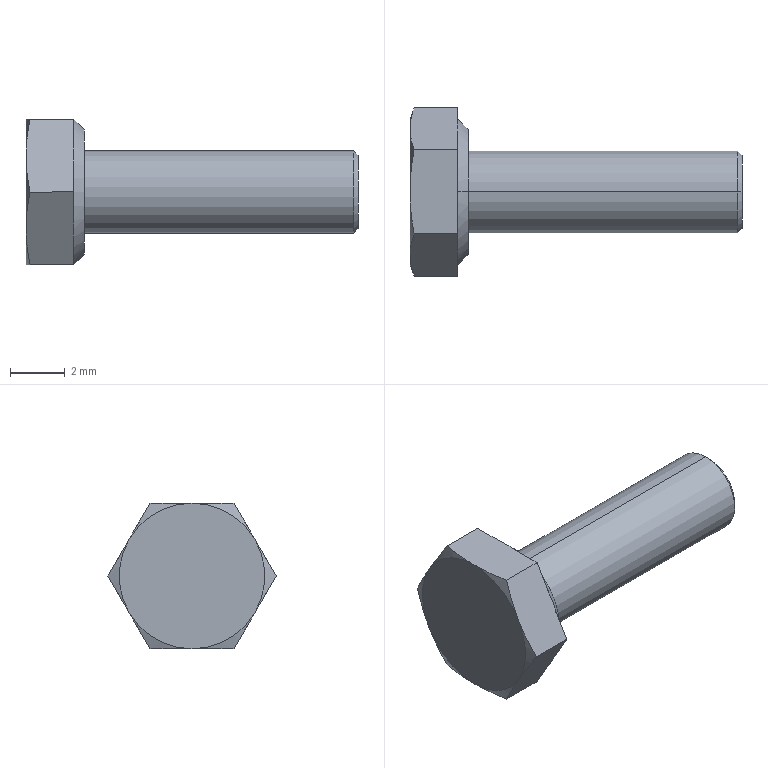Part | SolidWorks | features RevCut 3, Boss 1, Chamfer 1, Extrusion 1, Fillet 1, LPattern 1 | 1 solid | 27 faces | box 12.125 x 6.143 x 5.32 mm | volume 120.535 mm3 | plane 15 | cone 10 | cylinder 2 | commonest cylinder face diameters 3 x2
STEP:
#1=CARTESIAN_POINT('',(12.125,0.,-1.35));
#2=VERTEX_POINT('',#1);
#3=CARTESIAN_POINT('',(12.125,0.,1.35));
#4=VERTEX_POINT('',#3);
#5=CARTESIAN_POINT('',(12.125,0.,0.));
#6=DIRECTION('',(1.,0.,0.));
#7=DIRECTION('',(0.,0.,-1.));
#8=AXIS2_PLACEMENT_3D('',#5,#6,#7);
#9=CIRCLE('',#8,1.35);
#10=EDGE_CURVE('',#2,#4,#9,.T.);
#11=ORIENTED_EDGE('',*,*,#10,.F.);
#12=CARTESIAN_POINT('',(11.975,0.,-1.5));
#13=VERTEX_POINT('',#12);
#14=CARTESIAN_POINT('',(12.125,0.,-1.35));
#15=DIRECTION('',(-0.7071,0.,-0.7071));
#16=VECTOR('',#15,1000.);
#17=LINE('',#14,#16);
#18=EDGE_CURVE('',#2,#13,#17,.T.);
#19=ORIENTED_EDGE('',*,*,#18,.T.);
#20=CARTESIAN_POINT('',(11.975,0.,1.5));
#21=VERTEX_POINT('',#20);
#22=CARTESIAN_POINT('',(11.975,0.,0.));
#23=DIRECTION('',(-1.,0.,0.));
#24=DIRECTION('',(0.,0.,-1.));
#25=AXIS2_PLACEMENT_3D('',#22,#23,#24);
#26=CIRCLE('',#25,1.5);
#27=EDGE_CURVE('',#21,#13,#26,.T.);
#28=ORIENTED_EDGE('',*,*,#27,.F.);
#29=CARTESIAN_POINT('',(12.125,0.,1.35));
#30=DIRECTION('',(-0.7071,0.,0.7071));
#31=VECTOR('',#30,1000.);
#32=LINE('',#29,#31);
#33=EDGE_CURVE('',#4,#21,#32,.T.);
#34=ORIENTED_EDGE('',*,*,#33,.F.);
#35=EDGE_LOOP('',(#11,#19,#28,#34));
#36=FACE_OUTER_BOUND('',#35,.T.);
#37=CARTESIAN_POINT('',(12.125,0.,0.));
#38=DIRECTION('',(-1.,0.,0.));
#39=DIRECTION('',(0.,0.,1.));
#40=AXIS2_PLACEMENT_3D('',#37,#38,#39);
#41=CONICAL_SURFACE('',#40,1.35,0.7854);
#42=ADVANCED_FACE('',(#36),#41,.T.);
#43=ORIENTED_EDGE('',*,*,#27,.T.);
#44=CARTESIAN_POINT('',(2.125,0.,-1.5));
#45=VERTEX_POINT('',#44);
#46=CARTESIAN_POINT('',(12.125,0.,-1.5));
#47=DIRECTION('',(-1.,0.,0.));
#48=VECTOR('',#47,1000.);
#49=LINE('',#46,#48);
#50=EDGE_CURVE('',#13,#45,#49,.T.);
#51=ORIENTED_EDGE('',*,*,#50,.T.);
#52=CARTESIAN_POINT('',(2.125,0.,1.5));
#53=VERTEX_POINT('',#52);
#54=CARTESIAN_POINT('',(2.125,0.,0.));
#55=DIRECTION('',(1.,0.,0.));
#56=DIRECTION('',(0.,0.,-1.));
#57=AXIS2_PLACEMENT_3D('',#54,#55,#56);
#58=CIRCLE('',#57,1.5);
#59=EDGE_CURVE('',#45,#53,#58,.T.);
#60=ORIENTED_EDGE('',*,*,#59,.T.);
#61=CARTESIAN_POINT('',(12.125,0.,1.5));
#62=DIRECTION('',(-1.,0.,0.));
#63=VECTOR('',#62,1000.);
#64=LINE('',#61,#63);
#65=EDGE_CURVE('',#21,#53,#64,.T.);
#66=ORIENTED_EDGE('',*,*,#65,.F.);
#67=EDGE_LOOP('',(#43,#51,#60,#66));
#68=FACE_OUTER_BOUND('',#67,.T.);
#69=CARTESIAN_POINT('',(12.125,0.,0.));
#70=DIRECTION('',(-1.,0.,0.));
#71=DIRECTION('',(0.,0.,1.));
#72=AXIS2_PLACEMENT_3D('',#69,#70,#71);
#73=CYLINDRICAL_SURFACE('',#72,1.5);
#74=ADVANCED_FACE('',(#68),#73,.T.);
#75=CARTESIAN_POINT('',(2.125,0.,2.285));
#76=VERTEX_POINT('',#75);
#77=CARTESIAN_POINT('',(2.125,0.,-2.285));
#78=VERTEX_POINT('',#77);
#79=CARTESIAN_POINT('',(2.125,0.,0.));
#80=DIRECTION('',(-1.,0.,0.));
#81=DIRECTION('',(0.,0.,1.));
#82=AXIS2_PLACEMENT_3D('',#79,#80,#81);
#83=CIRCLE('',#82,2.285);
#84=EDGE_CURVE('',#76,#78,#83,.T.);
#85=ORIENTED_EDGE('',*,*,#84,.T.);
#86=CARTESIAN_POINT('',(1.75,0.,-2.66));
#87=VERTEX_POINT('',#86);
#88=CARTESIAN_POINT('',(1.725,0.,-2.685));
#89=DIRECTION('',(-0.7071,0.,-0.7071));
#90=VECTOR('',#89,1000.);
#91=LINE('',#88,#90);
#92=EDGE_CURVE('',#78,#87,#91,.T.);
#93=ORIENTED_EDGE('',*,*,#92,.T.);
#94=CARTESIAN_POINT('',(1.725,0.3655,-2.66));
#95=VERTEX_POINT('',#94);
#96=CARTESIAN_POINT('',(1.75,0.,-2.66));
#97=CARTESIAN_POINT('',(1.75,0.122,-2.66));
#98=CARTESIAN_POINT('',(1.742,0.2438,-2.66));
#99=CARTESIAN_POINT('',(1.725,0.3655,-2.66));
#100=B_SPLINE_CURVE_WITH_KNOTS('',3,(#96,#97,#98,#99),.UNSPECIFIED.,.F.,.F.,(4,4),(0.005987,0.006353),.UNSPECIFIED.);
#101=EDGE_CURVE('',#87,#95,#100,.T.);
#102=ORIENTED_EDGE('',*,*,#101,.T.);
#103=CARTESIAN_POINT('',(1.725,2.121,-1.647));
#104=VERTEX_POINT('',#103);
#105=CARTESIAN_POINT('',(1.725,0.,0.));
#106=DIRECTION('',(-1.,0.,0.));
#107=DIRECTION('',(0.,0.,1.));
#108=AXIS2_PLACEMENT_3D('',#105,#106,#107);
#109=CIRCLE('',#108,2.685);
#110=EDGE_CURVE('',#104,#95,#109,.T.);
#111=ORIENTED_EDGE('',*,*,#110,.F.);
#112=CARTESIAN_POINT('',(1.725,2.486,-1.013));
#113=VERTEX_POINT('',#112);
#114=CARTESIAN_POINT('',(1.725,2.121,-1.647));
#115=CARTESIAN_POINT('',(1.758,2.243,-1.436));
#116=CARTESIAN_POINT('',(1.758,2.365,-1.224));
#117=CARTESIAN_POINT('',(1.725,2.486,-1.013));
#118=B_SPLINE_CURVE_WITH_KNOTS('',3,(#114,#115,#116,#117),.UNSPECIFIED.,.F.,.F.,(4,4),(0.000001466,0.0007326),.UNSPECIFIED.);
#119=EDGE_CURVE('',#104,#113,#118,.T.);
#120=ORIENTED_EDGE('',*,*,#119,.T.);
#121=CARTESIAN_POINT('',(1.725,2.486,1.013));
#122=VERTEX_POINT('',#121);
#123=CARTESIAN_POINT('',(1.725,0.,0.));
#124=DIRECTION('',(-1.,0.,0.));
#125=DIRECTION('',(0.,0.,1.));
#126=AXIS2_PLACEMENT_3D('',#123,#124,#125);
#127=CIRCLE('',#126,2.685);
#128=EDGE_CURVE('',#122,#113,#127,.T.);
#129=ORIENTED_EDGE('',*,*,#128,.F.);
#130=CARTESIAN_POINT('',(1.725,2.121,1.647));
#131=VERTEX_POINT('',#130);
#132=CARTESIAN_POINT('',(1.725,2.486,1.013));
#133=CARTESIAN_POINT('',(1.758,2.365,1.224));
#134=CARTESIAN_POINT('',(1.758,2.243,1.436));
#135=CARTESIAN_POINT('',(1.725,2.121,1.647));
#136=B_SPLINE_CURVE_WITH_KNOTS('',3,(#132,#133,#134,#135),.UNSPECIFIED.,.F.,.F.,(4,4),(0.000001466,0.0007326),.UNSPECIFIED.);
#137=EDGE_CURVE('',#122,#131,#136,.T.);
#138=ORIENTED_EDGE('',*,*,#137,.T.);
#139=CARTESIAN_POINT('',(1.725,0.3655,2.66));
#140=VERTEX_POINT('',#139);
#141=CARTESIAN_POINT('',(1.725,0.,0.));
#142=DIRECTION('',(-1.,0.,0.));
#143=DIRECTION('',(0.,0.,1.));
#144=AXIS2_PLACEMENT_3D('',#141,#142,#143);
#145=CIRCLE('',#144,2.685);
#146=EDGE_CURVE('',#140,#131,#145,.T.);
#147=ORIENTED_EDGE('',*,*,#146,.F.);
#148=CARTESIAN_POINT('',(1.75,0.,2.66));
#149=VERTEX_POINT('',#148);
#150=CARTESIAN_POINT('',(1.725,0.3655,2.66));
#151=CARTESIAN_POINT('',(1.741,0.2453,2.66));
#152=CARTESIAN_POINT('',(1.75,0.1222,2.66));
#153=CARTESIAN_POINT('',(1.75,0.,2.66));
#154=B_SPLINE_CURVE_WITH_KNOTS('',3,(#150,#151,#152,#153),.UNSPECIFIED.,.F.,.F.,(4,4),(0.001277,0.001636),.UNSPECIFIED.);
#155=EDGE_CURVE('',#140,#149,#154,.T.);
#156=ORIENTED_EDGE('',*,*,#155,.T.);
#157=CARTESIAN_POINT('',(1.725,0.,2.685));
#158=DIRECTION('',(-0.7071,0.,0.7071));
#159=VECTOR('',#158,1000.);
#160=LINE('',#157,#159);
#161=EDGE_CURVE('',#76,#149,#160,.T.);
#162=ORIENTED_EDGE('',*,*,#161,.F.);
#163=EDGE_LOOP('',(#85,#93,#102,#111,#120,#129,#138,#147,#156,#162));
#164=FACE_OUTER_BOUND('',#163,.T.);
#165=CARTESIAN_POINT('',(1.725,0.,0.));
#166=DIRECTION('',(-1.,0.,0.));
#167=DIRECTION('',(0.,0.,1.));
#168=AXIS2_PLACEMENT_3D('',#165,#166,#167);
#169=CONICAL_SURFACE('',#168,2.685,0.7854);
#170=ADVANCED_FACE('',(#164),#169,.T.);
#171=ORIENTED_EDGE('',*,*,#84,.F.);
#172=CARTESIAN_POINT('',(2.125,0.,0.));
#173=DIRECTION('',(-1.,0.,0.));
#174=DIRECTION('',(0.,0.,1.));
#175=AXIS2_PLACEMENT_3D('',#172,#173,#174);
#176=CIRCLE('',#175,2.285);
#177=EDGE_CURVE('',#78,#76,#176,.T.);
#178=ORIENTED_EDGE('',*,*,#177,.F.);
#179=EDGE_LOOP('',(#171,#178));
#180=FACE_OUTER_BOUND('',#179,.T.);
#181=CARTESIAN_POINT('',(2.125,0.,0.));
#182=DIRECTION('',(1.,0.,0.));
#183=DIRECTION('',(0.,0.,-1.));
#184=AXIS2_PLACEMENT_3D('',#181,#182,#183);
#185=CIRCLE('',#184,1.5);
#186=EDGE_CURVE('',#53,#45,#185,.T.);
#187=ORIENTED_EDGE('',*,*,#186,.F.);
#188=ORIENTED_EDGE('',*,*,#59,.F.);
#189=EDGE_LOOP('',(#187,#188));
#190=FACE_BOUND('',#189,.T.);
#191=CARTESIAN_POINT('',(2.125,-1.536,-2.66));
#192=DIRECTION('',(1.,0.,0.));
#193=DIRECTION('',(0.,0.,-1.));
#194=AXIS2_PLACEMENT_3D('',#191,#192,#193);
#195=PLANE('',#194);
#196=ADVANCED_FACE('',(#180,#190),#195,.T.);
#197=CARTESIAN_POINT('',(0.1498,-1.536,-2.66));
#198=VERTEX_POINT('',#197);
#199=CARTESIAN_POINT('',(0.,-2.304,-1.33));
#200=VERTEX_POINT('',#199);
#201=CARTESIAN_POINT('',(0.1498,-1.536,-2.66));
#202=CARTESIAN_POINT('',(0.05661,-1.792,-2.217));
#203=CARTESIAN_POINT('',(0.,-2.048,-1.773));
#204=CARTESIAN_POINT('',(0.,-2.304,-1.33));
#205=B_SPLINE_CURVE_WITH_KNOTS('',3,(#201,#202,#203,#204),.UNSPECIFIED.,.F.,.F.,(4,4),(0.000000231,0.001536),.UNSPECIFIED.);
#206=EDGE_CURVE('',#198,#200,#205,.T.);
#207=ORIENTED_EDGE('',*,*,#206,.F.);
#208=CARTESIAN_POINT('',(1.725,-1.536,-2.66));
#209=VERTEX_POINT('',#208);
#210=CARTESIAN_POINT('',(2.125,-1.536,-2.66));
#211=DIRECTION('',(-1.,0.,0.));
#212=VECTOR('',#211,1000.);
#213=LINE('',#210,#212);
#214=EDGE_CURVE('',#209,#198,#213,.T.);
#215=ORIENTED_EDGE('',*,*,#214,.F.);
#216=CARTESIAN_POINT('',(1.725,-2.121,-1.647));
#217=VERTEX_POINT('',#216);
#218=CARTESIAN_POINT('',(1.725,-3.072,0.));
#219=DIRECTION('',(0.,0.5,-0.866));
#220=VECTOR('',#219,1000.);
#221=LINE('',#218,#220);
#222=EDGE_CURVE('',#217,#209,#221,.T.);
#223=ORIENTED_EDGE('',*,*,#222,.F.);
#224=CARTESIAN_POINT('',(1.725,-2.486,-1.013));
#225=VERTEX_POINT('',#224);
#226=CARTESIAN_POINT('',(1.725,-2.486,-1.013));
#227=CARTESIAN_POINT('',(1.758,-2.365,-1.224));
#228=CARTESIAN_POINT('',(1.758,-2.243,-1.436));
#229=CARTESIAN_POINT('',(1.725,-2.121,-1.647));
#230=B_SPLINE_CURVE_WITH_KNOTS('',3,(#226,#227,#228,#229),.UNSPECIFIED.,.F.,.F.,(4,4),(0.000001466,0.0007326),.UNSPECIFIED.);
#231=EDGE_CURVE('',#225,#217,#230,.T.);
#232=ORIENTED_EDGE('',*,*,#231,.F.);
#233=CARTESIAN_POINT('',(1.725,-3.072,0.));
#234=VERTEX_POINT('',#233);
#235=CARTESIAN_POINT('',(1.725,-3.072,0.));
#236=DIRECTION('',(0.,0.5,-0.866));
#237=VECTOR('',#236,1000.);
#238=LINE('',#235,#237);
#239=EDGE_CURVE('',#234,#225,#238,.T.);
#240=ORIENTED_EDGE('',*,*,#239,.F.);
#241=CARTESIAN_POINT('',(0.1498,-3.072,0.));
#242=VERTEX_POINT('',#241);
#243=CARTESIAN_POINT('',(2.125,-3.072,0.));
#244=DIRECTION('',(-1.,0.,0.));
#245=VECTOR('',#244,1000.);
#246=LINE('',#243,#245);
#247=EDGE_CURVE('',#234,#242,#246,.T.);
#248=ORIENTED_EDGE('',*,*,#247,.T.);
#249=CARTESIAN_POINT('',(0.,-2.304,-1.33));
#250=CARTESIAN_POINT('',(0.,-2.56,-0.8867));
#251=CARTESIAN_POINT('',(0.05661,-2.816,-0.4433));
#252=CARTESIAN_POINT('',(0.1498,-3.072,0.));
#253=B_SPLINE_CURVE_WITH_KNOTS('',3,(#249,#250,#251,#252),.UNSPECIFIED.,.F.,.F.,(4,4),(0.001536,0.003072),.UNSPECIFIED.);
#254=EDGE_CURVE('',#200,#242,#253,.T.);
#255=ORIENTED_EDGE('',*,*,#254,.F.);
#256=EDGE_LOOP('',(#207,#215,#223,#232,#240,#248,#255));
#257=FACE_OUTER_BOUND('',#256,.T.);
#258=CARTESIAN_POINT('',(2.125,-3.072,0.));
#259=DIRECTION('',(0.,0.866,0.5));
#260=DIRECTION('',(0.,-0.5,0.866));
#261=AXIS2_PLACEMENT_3D('',#258,#259,#260);
#262=PLANE('',#261);
#263=ADVANCED_FACE('',(#257),#262,.F.);
#264=CARTESIAN_POINT('',(0.1498,1.536,-2.66));
#265=VERTEX_POINT('',#264);
#266=CARTESIAN_POINT('',(0.,0.,-2.66));
#267=VERTEX_POINT('',#266);
#268=CARTESIAN_POINT('',(0.1498,1.536,-2.66));
#269=CARTESIAN_POINT('',(0.05687,1.025,-2.66));
#270=CARTESIAN_POINT('',(0.,0.513,-2.66));
#271=CARTESIAN_POINT('',(0.,0.,-2.66));
#272=B_SPLINE_CURVE_WITH_KNOTS('',3,(#268,#269,#270,#271),.UNSPECIFIED.,.F.,.F.,(4,4),(0.005538,0.007086),.UNSPECIFIED.);
#273=EDGE_CURVE('',#265,#267,#272,.T.);
#274=ORIENTED_EDGE('',*,*,#273,.F.);
#275=CARTESIAN_POINT('',(1.725,1.536,-2.66));
#276=VERTEX_POINT('',#275);
#277=CARTESIAN_POINT('',(2.125,1.536,-2.66));
#278=DIRECTION('',(-1.,0.,0.));
#279=VECTOR('',#278,1000.);
#280=LINE('',#277,#279);
#281=EDGE_CURVE('',#276,#265,#280,.T.);
#282=ORIENTED_EDGE('',*,*,#281,.F.);
#283=CARTESIAN_POINT('',(1.725,-1.536,-2.66));
#284=DIRECTION('',(0.,1.,0.));
#285=VECTOR('',#284,1000.);
#286=LINE('',#283,#285);
#287=EDGE_CURVE('',#95,#276,#286,.T.);
#288=ORIENTED_EDGE('',*,*,#287,.F.);
#289=ORIENTED_EDGE('',*,*,#101,.F.);
#290=CARTESIAN_POINT('',(1.725,-0.3655,-2.66));
#291=VERTEX_POINT('',#290);
#292=CARTESIAN_POINT('',(1.725,-0.3655,-2.66));
#293=CARTESIAN_POINT('',(1.742,-0.2437,-2.66));
#294=CARTESIAN_POINT('',(1.75,-0.1217,-2.66));
#295=CARTESIAN_POINT('',(1.75,0.,-2.66));
#296=B_SPLINE_CURVE_WITH_KNOTS('',3,(#292,#293,#294,#295),.UNSPECIFIED.,.F.,.F.,(4,4),(0.005622,0.005987),.UNSPECIFIED.);
#297=EDGE_CURVE('',#291,#87,#296,.T.);
#298=ORIENTED_EDGE('',*,*,#297,.F.);
#299=CARTESIAN_POINT('',(1.725,-1.536,-2.66));
#300=DIRECTION('',(0.,1.,0.));
#301=VECTOR('',#300,1000.);
#302=LINE('',#299,#301);
#303=EDGE_CURVE('',#209,#291,#302,.T.);
#304=ORIENTED_EDGE('',*,*,#303,.F.);
#305=ORIENTED_EDGE('',*,*,#214,.T.);
#306=CARTESIAN_POINT('',(0.,0.,-2.66));
#307=CARTESIAN_POINT('',(0.,-0.2558,-2.66));
#308=CARTESIAN_POINT('',(0.01368,-0.5118,-2.66));
#309=CARTESIAN_POINT('',(0.06543,-1.024,-2.66));
#310=CARTESIAN_POINT('',(0.1035,-1.281,-2.66));
#311=CARTESIAN_POINT('',(0.1498,-1.536,-2.66));
#312=B_SPLINE_CURVE_WITH_KNOTS('',3,(#306,#307,#308,#309,#310,#311),.UNSPECIFIED.,.F.,.F.,(4,2,4),(0.007086,0.007858,0.00863),.UNSPECIFIED.);
#313=EDGE_CURVE('',#267,#198,#312,.T.);
#314=ORIENTED_EDGE('',*,*,#313,.F.);
#315=EDGE_LOOP('',(#274,#282,#288,#289,#298,#304,#305,#314));
#316=FACE_OUTER_BOUND('',#315,.T.);
#317=CARTESIAN_POINT('',(2.125,-1.536,-2.66));
#318=DIRECTION('',(0.,0.,1.));
#319=DIRECTION('',(0.,-1.,0.));
#320=AXIS2_PLACEMENT_3D('',#317,#318,#319);
#321=PLANE('',#320);
#322=ADVANCED_FACE('',(#316),#321,.F.);
#323=CARTESIAN_POINT('',(0.1498,3.072,0.));
#324=VERTEX_POINT('',#323);
#325=CARTESIAN_POINT('',(0.,2.304,-1.33));
#326=VERTEX_POINT('',#325);
#327=CARTESIAN_POINT('',(0.1498,3.072,0.));
#328=CARTESIAN_POINT('',(0.05661,2.816,-0.4433));
#329=CARTESIAN_POINT('',(0.,2.56,-0.8867));
#330=CARTESIAN_POINT('',(0.,2.304,-1.33));
#331=B_SPLINE_CURVE_WITH_KNOTS('',3,(#327,#328,#329,#330),.UNSPECIFIED.,.F.,.F.,(4,4),(0.000000231,0.001536),.UNSPECIFIED.);
#332=EDGE_CURVE('',#324,#326,#331,.T.);
#333=ORIENTED_EDGE('',*,*,#332,.F.);
#334=CARTESIAN_POINT('',(1.725,3.072,0.));
#335=VERTEX_POINT('',#334);
#336=CARTESIAN_POINT('',(2.125,3.072,0.));
#337=DIRECTION('',(-1.,0.,0.));
#338=VECTOR('',#337,1000.);
#339=LINE('',#336,#338);
#340=EDGE_CURVE('',#335,#324,#339,.T.);
#341=ORIENTED_EDGE('',*,*,#340,.F.);
#342=CARTESIAN_POINT('',(1.725,1.536,-2.66));
#343=DIRECTION('',(0.,0.5,0.866));
#344=VECTOR('',#343,1000.);
#345=LINE('',#342,#344);
#346=EDGE_CURVE('',#113,#335,#345,.T.);
#347=ORIENTED_EDGE('',*,*,#346,.F.);
#348=ORIENTED_EDGE('',*,*,#119,.F.);
#349=CARTESIAN_POINT('',(1.725,1.536,-2.66));
#350=DIRECTION('',(0.,0.5,0.866));
#351=VECTOR('',#350,1000.);
#352=LINE('',#349,#351);
#353=EDGE_CURVE('',#276,#104,#352,.T.);
#354=ORIENTED_EDGE('',*,*,#353,.F.);
#355=ORIENTED_EDGE('',*,*,#281,.T.);
#356=CARTESIAN_POINT('',(0.,2.304,-1.33));
#357=CARTESIAN_POINT('',(0.,2.048,-1.773));
#358=CARTESIAN_POINT('',(0.05661,1.792,-2.217));
#359=CARTESIAN_POINT('',(0.1498,1.536,-2.66));
#360=B_SPLINE_CURVE_WITH_KNOTS('',3,(#356,#357,#358,#359),.UNSPECIFIED.,.F.,.F.,(4,4),(0.001536,0.003072),.UNSPECIFIED.);
#361=EDGE_CURVE('',#326,#265,#360,.T.);
#362=ORIENTED_EDGE('',*,*,#361,.F.);
#363=EDGE_LOOP('',(#333,#341,#347,#348,#354,#355,#362));
#364=FACE_OUTER_BOUND('',#363,.T.);
#365=CARTESIAN_POINT('',(2.125,1.536,-2.66));
#366=DIRECTION('',(0.,-0.866,0.5));
#367=DIRECTION('',(0.,-0.5,-0.866));
#368=AXIS2_PLACEMENT_3D('',#365,#366,#367);
#369=PLANE('',#368);
#370=ADVANCED_FACE('',(#364),#369,.F.);
#371=CARTESIAN_POINT('',(0.1498,1.536,2.66));
#372=VERTEX_POINT('',#371);
#373=CARTESIAN_POINT('',(0.,2.304,1.33));
#374=VERTEX_POINT('',#373);
#375=CARTESIAN_POINT('',(0.1498,1.536,2.66));
#376=CARTESIAN_POINT('',(0.05661,1.792,2.217));
#377=CARTESIAN_POINT('',(0.,2.048,1.773));
#378=CARTESIAN_POINT('',(0.,2.304,1.33));
#379=B_SPLINE_CURVE_WITH_KNOTS('',3,(#375,#376,#377,#378),.UNSPECIFIED.,.F.,.F.,(4,4),(0.000000231,0.001536),.UNSPECIFIED.);
#380=EDGE_CURVE('',#372,#374,#379,.T.);
#381=ORIENTED_EDGE('',*,*,#380,.F.);
#382=CARTESIAN_POINT('',(1.725,1.536,2.66));
#383=VERTEX_POINT('',#382);
#384=CARTESIAN_POINT('',(2.125,1.536,2.66));
#385=DIRECTION('',(-1.,0.,0.));
#386=VECTOR('',#385,1000.);
#387=LINE('',#384,#386);
#388=EDGE_CURVE('',#383,#372,#387,.T.);
#389=ORIENTED_EDGE('',*,*,#388,.F.);
#390=CARTESIAN_POINT('',(1.725,3.072,0.));
#391=DIRECTION('',(0.,-0.5,0.866));
#392=VECTOR('',#391,1000.);
#393=LINE('',#390,#392);
#394=EDGE_CURVE('',#131,#383,#393,.T.);
#395=ORIENTED_EDGE('',*,*,#394,.F.);
#396=ORIENTED_EDGE('',*,*,#137,.F.);
#397=CARTESIAN_POINT('',(1.725,3.072,0.));
#398=DIRECTION('',(0.,-0.5,0.866));
#399=VECTOR('',#398,1000.);
#400=LINE('',#397,#399);
#401=EDGE_CURVE('',#335,#122,#400,.T.);
#402=ORIENTED_EDGE('',*,*,#401,.F.);
#403=ORIENTED_EDGE('',*,*,#340,.T.);
#404=CARTESIAN_POINT('',(0.,2.304,1.33));
#405=CARTESIAN_POINT('',(0.,2.56,0.8867));
#406=CARTESIAN_POINT('',(0.05661,2.816,0.4433));
#407=CARTESIAN_POINT('',(0.1498,3.072,0.));
#408=B_SPLINE_CURVE_WITH_KNOTS('',3,(#404,#405,#406,#407),.UNSPECIFIED.,.F.,.F.,(4,4),(0.001536,0.003072),.UNSPECIFIED.);
#409=EDGE_CURVE('',#374,#324,#408,.T.);
#410=ORIENTED_EDGE('',*,*,#409,.F.);
#411=EDGE_LOOP('',(#381,#389,#395,#396,#402,#403,#410));
#412=FACE_OUTER_BOUND('',#411,.T.);
#413=CARTESIAN_POINT('',(2.125,3.072,0.));
#414=DIRECTION('',(0.,-0.866,-0.5));
#415=DIRECTION('',(0.,0.5,-0.866));
#416=AXIS2_PLACEMENT_3D('',#413,#414,#415);
#417=PLANE('',#416);
#418=ADVANCED_FACE('',(#412),#417,.F.);
#419=CARTESIAN_POINT('',(0.1498,-1.536,2.66));
#420=VERTEX_POINT('',#419);
#421=CARTESIAN_POINT('',(0.,0.,2.66));
#422=VERTEX_POINT('',#421);
#423=CARTESIAN_POINT('',(0.1498,-1.536,2.66));
#424=CARTESIAN_POINT('',(0.1035,-1.281,2.66));
#425=CARTESIAN_POINT('',(0.06543,-1.024,2.66));
#426=CARTESIAN_POINT('',(0.01368,-0.5118,2.66));
#427=CARTESIAN_POINT('',(0.,-0.2558,2.66));
#428=CARTESIAN_POINT('',(0.,0.,2.66));
#429=B_SPLINE_CURVE_WITH_KNOTS('',3,(#423,#424,#425,#426,#427,#428),.UNSPECIFIED.,.F.,.F.,(4,2,4),(0.002612,0.003386,0.00416),.UNSPECIFIED.);
#430=EDGE_CURVE('',#420,#422,#429,.T.);
#431=ORIENTED_EDGE('',*,*,#430,.F.);
#432=CARTESIAN_POINT('',(1.725,-1.536,2.66));
#433=VERTEX_POINT('',#432);
#434=CARTESIAN_POINT('',(2.125,-1.536,2.66));
#435=DIRECTION('',(-1.,0.,0.));
#436=VECTOR('',#435,1000.);
#437=LINE('',#434,#436);
#438=EDGE_CURVE('',#433,#420,#437,.T.);
#439=ORIENTED_EDGE('',*,*,#438,.F.);
#440=CARTESIAN_POINT('',(1.725,-0.3655,2.66));
#441=VERTEX_POINT('',#440);
#442=CARTESIAN_POINT('',(1.725,1.536,2.66));
#443=DIRECTION('',(0.,-1.,0.));
#444=VECTOR('',#443,1000.);
#445=LINE('',#442,#444);
#446=EDGE_CURVE('',#441,#433,#445,.T.);
#447=ORIENTED_EDGE('',*,*,#446,.F.);
#448=CARTESIAN_POINT('',(1.75,0.,2.66));
#449=CARTESIAN_POINT('',(1.75,-0.1221,2.66));
#450=CARTESIAN_POINT('',(1.742,-0.2441,2.66));
#451=CARTESIAN_POINT('',(1.725,-0.3655,2.66));
#452=B_SPLINE_CURVE_WITH_KNOTS('',3,(#448,#449,#450,#451),.UNSPECIFIED.,.F.,.F.,(4,4),(0.001636,0.001994),.UNSPECIFIED.);
#453=EDGE_CURVE('',#149,#441,#452,.T.);
#454=ORIENTED_EDGE('',*,*,#453,.F.);
#455=ORIENTED_EDGE('',*,*,#155,.F.);
#456=CARTESIAN_POINT('',(1.725,1.536,2.66));
#457=DIRECTION('',(0.,-1.,0.));
#458=VECTOR('',#457,1000.);
#459=LINE('',#456,#458);
#460=EDGE_CURVE('',#383,#140,#459,.T.);
#461=ORIENTED_EDGE('',*,*,#460,.F.);
#462=ORIENTED_EDGE('',*,*,#388,.T.);
#463=CARTESIAN_POINT('',(0.,0.,2.66));
#464=CARTESIAN_POINT('',(0.,0.513,2.66));
#465=CARTESIAN_POINT('',(0.05687,1.025,2.66));
#466=CARTESIAN_POINT('',(0.1498,1.536,2.66));
#467=B_SPLINE_CURVE_WITH_KNOTS('',3,(#463,#464,#465,#466),.UNSPECIFIED.,.F.,.F.,(4,4),(0.00416,0.005713),.UNSPECIFIED.);
#468=EDGE_CURVE('',#422,#372,#467,.T.);
#469=ORIENTED_EDGE('',*,*,#468,.F.);
#470=EDGE_LOOP('',(#431,#439,#447,#454,#455,#461,#462,#469));
#471=FACE_OUTER_BOUND('',#470,.T.);
#472=CARTESIAN_POINT('',(2.125,1.536,2.66));
#473=DIRECTION('',(0.,0.,-1.));
#474=DIRECTION('',(0.,1.,0.));
#475=AXIS2_PLACEMENT_3D('',#472,#473,#474);
#476=PLANE('',#475);
#477=ADVANCED_FACE('',(#471),#476,.F.);
#478=CARTESIAN_POINT('',(0.,-2.304,1.33));
#479=VERTEX_POINT('',#478);
#480=CARTESIAN_POINT('',(0.1498,-3.072,0.));
#481=CARTESIAN_POINT('',(0.05661,-2.816,0.4433));
#482=CARTESIAN_POINT('',(0.,-2.56,0.8867));
#483=CARTESIAN_POINT('',(0.,-2.304,1.33));
#484=B_SPLINE_CURVE_WITH_KNOTS('',3,(#480,#481,#482,#483),.UNSPECIFIED.,.F.,.F.,(4,4),(0.000000231,0.001536),.UNSPECIFIED.);
#485=EDGE_CURVE('',#242,#479,#484,.T.);
#486=ORIENTED_EDGE('',*,*,#485,.F.);
#487=ORIENTED_EDGE('',*,*,#247,.F.);
#488=CARTESIAN_POINT('',(1.725,-2.486,1.013));
#489=VERTEX_POINT('',#488);
#490=CARTESIAN_POINT('',(1.725,-1.536,2.66));
#491=DIRECTION('',(0.,-0.5,-0.866));
#492=VECTOR('',#491,1000.);
#493=LINE('',#490,#492);
#494=EDGE_CURVE('',#489,#234,#493,.T.);
#495=ORIENTED_EDGE('',*,*,#494,.F.);
#496=CARTESIAN_POINT('',(1.725,-2.121,1.647));
#497=VERTEX_POINT('',#496);
#498=CARTESIAN_POINT('',(1.725,-2.121,1.647));
#499=CARTESIAN_POINT('',(1.758,-2.243,1.436));
#500=CARTESIAN_POINT('',(1.758,-2.365,1.224));
#501=CARTESIAN_POINT('',(1.725,-2.486,1.013));
#502=B_SPLINE_CURVE_WITH_KNOTS('',3,(#498,#499,#500,#501),.UNSPECIFIED.,.F.,.F.,(4,4),(0.000001466,0.0007326),.UNSPECIFIED.);
#503=EDGE_CURVE('',#497,#489,#502,.T.);
#504=ORIENTED_EDGE('',*,*,#503,.F.);
#505=CARTESIAN_POINT('',(1.725,-1.536,2.66));
#506=DIRECTION('',(0.,-0.5,-0.866));
#507=VECTOR('',#506,1000.);
#508=LINE('',#505,#507);
#509=EDGE_CURVE('',#433,#497,#508,.T.);
#510=ORIENTED_EDGE('',*,*,#509,.F.);
#511=ORIENTED_EDGE('',*,*,#438,.T.);
#512=CARTESIAN_POINT('',(0.,-2.304,1.33));
#513=CARTESIAN_POINT('',(0.,-2.048,1.773));
#514=CARTESIAN_POINT('',(0.05661,-1.792,2.217));
#515=CARTESIAN_POINT('',(0.1498,-1.536,2.66));
#516=B_SPLINE_CURVE_WITH_KNOTS('',3,(#512,#513,#514,#515),.UNSPECIFIED.,.F.,.F.,(4,4),(0.001536,0.003072),.UNSPECIFIED.);
#517=EDGE_CURVE('',#479,#420,#516,.T.);
#518=ORIENTED_EDGE('',*,*,#517,.F.);
#519=EDGE_LOOP('',(#486,#487,#495,#504,#510,#511,#518));
#520=FACE_OUTER_BOUND('',#519,.T.);
#521=CARTESIAN_POINT('',(2.125,-1.536,2.66));
#522=DIRECTION('',(0.,0.866,-0.5));
#523=DIRECTION('',(0.,0.5,0.866));
#524=AXIS2_PLACEMENT_3D('',#521,#522,#523);
#525=PLANE('',#524);
#526=ADVANCED_FACE('',(#520),#525,.F.);
#527=ORIENTED_EDGE('',*,*,#222,.T.);
#528=ORIENTED_EDGE('',*,*,#303,.T.);
#529=CARTESIAN_POINT('',(1.725,0.,0.));
#530=DIRECTION('',(-1.,0.,0.));
#531=DIRECTION('',(0.,0.,1.));
#532=AXIS2_PLACEMENT_3D('',#529,#530,#531);
#533=CIRCLE('',#532,2.685);
#534=EDGE_CURVE('',#291,#217,#533,.T.);
#535=ORIENTED_EDGE('',*,*,#534,.T.);
#536=EDGE_LOOP('',(#527,#528,#535));
#537=FACE_OUTER_BOUND('',#536,.T.);
#538=CARTESIAN_POINT('',(1.725,2.685,0.));
#539=DIRECTION('',(1.,0.,0.));
#540=DIRECTION('',(0.,0.,-1.));
#541=AXIS2_PLACEMENT_3D('',#538,#539,#540);
#542=PLANE('',#541);
#543=ADVANCED_FACE('',(#537),#542,.T.);
#544=ORIENTED_EDGE('',*,*,#287,.T.);
#545=ORIENTED_EDGE('',*,*,#353,.T.);
#546=ORIENTED_EDGE('',*,*,#110,.T.);
#547=EDGE_LOOP('',(#544,#545,#546));
#548=FACE_OUTER_BOUND('',#547,.T.);
#549=CARTESIAN_POINT('',(1.725,2.685,0.));
#550=DIRECTION('',(1.,0.,0.));
#551=DIRECTION('',(0.,0.,-1.));
#552=AXIS2_PLACEMENT_3D('',#549,#550,#551);
#553=PLANE('',#552);
#554=ADVANCED_FACE('',(#548),#553,.T.);
#555=ORIENTED_EDGE('',*,*,#346,.T.);
#556=ORIENTED_EDGE('',*,*,#401,.T.);
#557=ORIENTED_EDGE('',*,*,#128,.T.);
#558=EDGE_LOOP('',(#555,#556,#557));
#559=FACE_OUTER_BOUND('',#558,.T.);
#560=CARTESIAN_POINT('',(1.725,2.685,0.));
#561=DIRECTION('',(1.,0.,0.));
#562=DIRECTION('',(0.,0.,-1.));
#563=AXIS2_PLACEMENT_3D('',#560,#561,#562);
#564=PLANE('',#563);
#565=ADVANCED_FACE('',(#559),#564,.T.);
#566=ORIENTED_EDGE('',*,*,#394,.T.);
#567=ORIENTED_EDGE('',*,*,#460,.T.);
#568=ORIENTED_EDGE('',*,*,#146,.T.);
#569=EDGE_LOOP('',(#566,#567,#568));
#570=FACE_OUTER_BOUND('',#569,.T.);
#571=CARTESIAN_POINT('',(1.725,2.685,0.));
#572=DIRECTION('',(1.,0.,0.));
#573=DIRECTION('',(0.,0.,-1.));
#574=AXIS2_PLACEMENT_3D('',#571,#572,#573);
#575=PLANE('',#574);
#576=ADVANCED_FACE('',(#570),#575,.T.);
#577=ORIENTED_EDGE('',*,*,#446,.T.);
#578=ORIENTED_EDGE('',*,*,#509,.T.);
#579=CARTESIAN_POINT('',(1.725,0.,0.));
#580=DIRECTION('',(-1.,0.,0.));
#581=DIRECTION('',(0.,0.,1.));
#582=AXIS2_PLACEMENT_3D('',#579,#580,#581);
#583=CIRCLE('',#582,2.685);
#584=EDGE_CURVE('',#497,#441,#583,.T.);
#585=ORIENTED_EDGE('',*,*,#584,.T.);
#586=EDGE_LOOP('',(#577,#578,#585));
#587=FACE_OUTER_BOUND('',#586,.T.);
#588=CARTESIAN_POINT('',(1.725,2.685,0.));
#589=DIRECTION('',(1.,0.,0.));
#590=DIRECTION('',(0.,0.,-1.));
#591=AXIS2_PLACEMENT_3D('',#588,#589,#590);
#592=PLANE('',#591);
#593=ADVANCED_FACE('',(#587),#592,.T.);
#594=ORIENTED_EDGE('',*,*,#239,.T.);
#595=CARTESIAN_POINT('',(1.725,0.,0.));
#596=DIRECTION('',(-1.,0.,0.));
#597=DIRECTION('',(0.,0.,1.));
#598=AXIS2_PLACEMENT_3D('',#595,#596,#597);
#599=CIRCLE('',#598,2.685);
#600=EDGE_CURVE('',#225,#489,#599,.T.);
#601=ORIENTED_EDGE('',*,*,#600,.T.);
#602=ORIENTED_EDGE('',*,*,#494,.T.);
#603=EDGE_LOOP('',(#594,#601,#602));
#604=FACE_OUTER_BOUND('',#603,.T.);
#605=CARTESIAN_POINT('',(1.725,2.685,0.));
#606=DIRECTION('',(1.,0.,0.));
#607=DIRECTION('',(0.,0.,-1.));
#608=AXIS2_PLACEMENT_3D('',#605,#606,#607);
#609=PLANE('',#608);
#610=ADVANCED_FACE('',(#604),#609,.T.);
#611=ORIENTED_EDGE('',*,*,#92,.F.);
#612=ORIENTED_EDGE('',*,*,#177,.T.);
#613=ORIENTED_EDGE('',*,*,#161,.T.);
#614=ORIENTED_EDGE('',*,*,#453,.T.);
#615=ORIENTED_EDGE('',*,*,#584,.F.);
#616=ORIENTED_EDGE('',*,*,#503,.T.);
#617=ORIENTED_EDGE('',*,*,#600,.F.);
#618=ORIENTED_EDGE('',*,*,#231,.T.);
#619=ORIENTED_EDGE('',*,*,#534,.F.);
#620=ORIENTED_EDGE('',*,*,#297,.T.);
#621=EDGE_LOOP('',(#611,#612,#613,#614,#615,#616,#617,#618,#619,#620));
#622=FACE_OUTER_BOUND('',#621,.T.);
#623=CARTESIAN_POINT('',(1.725,0.,0.));
#624=DIRECTION('',(-1.,0.,0.));
#625=DIRECTION('',(0.,0.,1.));
#626=AXIS2_PLACEMENT_3D('',#623,#624,#625);
#627=CONICAL_SURFACE('',#626,2.685,0.7854);
#628=ADVANCED_FACE('',(#622),#627,.T.);
#629=ORIENTED_EDGE('',*,*,#313,.T.);
#630=ORIENTED_EDGE('',*,*,#206,.T.);
#631=CARTESIAN_POINT('',(0.,0.,0.));
#632=DIRECTION('',(1.,0.,0.));
#633=DIRECTION('',(0.,0.,-1.));
#634=AXIS2_PLACEMENT_3D('',#631,#632,#633);
#635=CIRCLE('',#634,2.66);
#636=EDGE_CURVE('',#200,#267,#635,.T.);
#637=ORIENTED_EDGE('',*,*,#636,.T.);
#638=EDGE_LOOP('',(#629,#630,#637));
#639=FACE_OUTER_BOUND('',#638,.T.);
#640=CARTESIAN_POINT('',(0.,0.,0.));
#641=DIRECTION('',(1.,0.,0.));
#642=DIRECTION('',(0.,0.,-1.));
#643=AXIS2_PLACEMENT_3D('',#640,#641,#642);
#644=CONICAL_SURFACE('',#643,2.66,1.222);
#645=ADVANCED_FACE('',(#639),#644,.T.);
#646=ORIENTED_EDGE('',*,*,#254,.T.);
#647=ORIENTED_EDGE('',*,*,#485,.T.);
#648=CARTESIAN_POINT('',(0.,0.,0.));
#649=DIRECTION('',(1.,0.,0.));
#650=DIRECTION('',(0.,0.,-1.));
#651=AXIS2_PLACEMENT_3D('',#648,#649,#650);
#652=CIRCLE('',#651,2.66);
#653=EDGE_CURVE('',#479,#200,#652,.T.);
#654=ORIENTED_EDGE('',*,*,#653,.T.);
#655=EDGE_LOOP('',(#646,#647,#654));
#656=FACE_OUTER_BOUND('',#655,.T.);
#657=CARTESIAN_POINT('',(0.,0.,0.));
#658=DIRECTION('',(1.,0.,0.));
#659=DIRECTION('',(0.,0.,-1.));
#660=AXIS2_PLACEMENT_3D('',#657,#658,#659);
#661=CONICAL_SURFACE('',#660,2.66,1.222);
#662=ADVANCED_FACE('',(#656),#661,.T.);
#663=ORIENTED_EDGE('',*,*,#430,.T.);
#664=CARTESIAN_POINT('',(0.,0.,0.));
#665=DIRECTION('',(1.,0.,0.));
#666=DIRECTION('',(0.,0.,-1.));
#667=AXIS2_PLACEMENT_3D('',#664,#665,#666);
#668=CIRCLE('',#667,2.66);
#669=EDGE_CURVE('',#422,#479,#668,.T.);
#670=ORIENTED_EDGE('',*,*,#669,.T.);
#671=ORIENTED_EDGE('',*,*,#517,.T.);
#672=EDGE_LOOP('',(#663,#670,#671));
#673=FACE_OUTER_BOUND('',#672,.T.);
#674=CARTESIAN_POINT('',(0.,0.,0.));
#675=DIRECTION('',(1.,0.,0.));
#676=DIRECTION('',(0.,0.,-1.));
#677=AXIS2_PLACEMENT_3D('',#674,#675,#676);
#678=CONICAL_SURFACE('',#677,2.66,1.222);
#679=ADVANCED_FACE('',(#673),#678,.T.);
#680=ORIENTED_EDGE('',*,*,#380,.T.);
#681=CARTESIAN_POINT('',(0.,0.,0.));
#682=DIRECTION('',(-1.,0.,0.));
#683=DIRECTION('',(0.,0.,1.));
#684=AXIS2_PLACEMENT_3D('',#681,#682,#683);
#685=CIRCLE('',#684,2.66);
#686=EDGE_CURVE('',#422,#374,#685,.T.);
#687=ORIENTED_EDGE('',*,*,#686,.F.);
#688=ORIENTED_EDGE('',*,*,#468,.T.);
#689=EDGE_LOOP('',(#680,#687,#688));
#690=FACE_OUTER_BOUND('',#689,.T.);
#691=CARTESIAN_POINT('',(0.,0.,0.));
#692=DIRECTION('',(1.,0.,0.));
#693=DIRECTION('',(0.,0.,-1.));
#694=AXIS2_PLACEMENT_3D('',#691,#692,#693);
#695=CONICAL_SURFACE('',#694,2.66,1.222);
#696=ADVANCED_FACE('',(#690),#695,.T.);
#697=ORIENTED_EDGE('',*,*,#332,.T.);
#698=CARTESIAN_POINT('',(0.,0.,0.));
#699=DIRECTION('',(1.,0.,0.));
#700=DIRECTION('',(0.,0.,-1.));
#701=AXIS2_PLACEMENT_3D('',#698,#699,#700);
#702=CIRCLE('',#701,2.66);
#703=EDGE_CURVE('',#326,#374,#702,.T.);
#704=ORIENTED_EDGE('',*,*,#703,.T.);
#705=ORIENTED_EDGE('',*,*,#409,.T.);
#706=EDGE_LOOP('',(#697,#704,#705));
#707=FACE_OUTER_BOUND('',#706,.T.);
#708=CARTESIAN_POINT('',(0.,0.,0.));
#709=DIRECTION('',(1.,0.,0.));
#710=DIRECTION('',(0.,0.,-1.));
#711=AXIS2_PLACEMENT_3D('',#708,#709,#710);
#712=CONICAL_SURFACE('',#711,2.66,1.222);
#713=ADVANCED_FACE('',(#707),#712,.T.);
#714=ORIENTED_EDGE('',*,*,#361,.T.);
#715=ORIENTED_EDGE('',*,*,#273,.T.);
#716=CARTESIAN_POINT('',(0.,0.,0.));
#717=DIRECTION('',(1.,0.,0.));
#718=DIRECTION('',(0.,0.,-1.));
#719=AXIS2_PLACEMENT_3D('',#716,#717,#718);
#720=CIRCLE('',#719,2.66);
#721=EDGE_CURVE('',#267,#326,#720,.T.);
#722=ORIENTED_EDGE('',*,*,#721,.T.);
#723=EDGE_LOOP('',(#714,#715,#722));
#724=FACE_OUTER_BOUND('',#723,.T.);
#725=CARTESIAN_POINT('',(0.,0.,0.));
#726=DIRECTION('',(1.,0.,0.));
#727=DIRECTION('',(0.,0.,-1.));
#728=AXIS2_PLACEMENT_3D('',#725,#726,#727);
#729=CONICAL_SURFACE('',#728,2.66,1.222);
#730=ADVANCED_FACE('',(#724),#729,.T.);
#731=ORIENTED_EDGE('',*,*,#721,.F.);
#732=ORIENTED_EDGE('',*,*,#636,.F.);
#733=ORIENTED_EDGE('',*,*,#653,.F.);
#734=ORIENTED_EDGE('',*,*,#669,.F.);
#735=ORIENTED_EDGE('',*,*,#686,.T.);
#736=ORIENTED_EDGE('',*,*,#703,.F.);
#737=EDGE_LOOP('',(#731,#732,#733,#734,#735,#736));
#738=FACE_OUTER_BOUND('',#737,.T.);
#739=CARTESIAN_POINT('',(0.,-1.536,-2.66));
#740=DIRECTION('',(1.,0.,0.));
#741=DIRECTION('',(0.,0.,-1.));
#742=AXIS2_PLACEMENT_3D('',#739,#740,#741);
#743=PLANE('',#742);
#744=ADVANCED_FACE('',(#738),#743,.F.);
#745=ORIENTED_EDGE('',*,*,#50,.F.);
#746=CARTESIAN_POINT('',(11.975,0.,0.));
#747=DIRECTION('',(-1.,0.,0.));
#748=DIRECTION('',(0.,0.,-1.));
#749=AXIS2_PLACEMENT_3D('',#746,#747,#748);
#750=CIRCLE('',#749,1.5);
#751=EDGE_CURVE('',#13,#21,#750,.T.);
#752=ORIENTED_EDGE('',*,*,#751,.T.);
#753=ORIENTED_EDGE('',*,*,#65,.T.);
#754=ORIENTED_EDGE('',*,*,#186,.T.);
#755=EDGE_LOOP('',(#745,#752,#753,#754));
#756=FACE_OUTER_BOUND('',#755,.T.);
#757=CARTESIAN_POINT('',(12.125,0.,0.));
#758=DIRECTION('',(-1.,0.,0.));
#759=DIRECTION('',(0.,0.,1.));
#760=AXIS2_PLACEMENT_3D('',#757,#758,#759);
#761=CYLINDRICAL_SURFACE('',#760,1.5);
#762=ADVANCED_FACE('',(#756),#761,.T.);
#763=CARTESIAN_POINT('',(12.125,0.,0.));
#764=DIRECTION('',(1.,0.,0.));
#765=DIRECTION('',(0.,0.,-1.));
#766=AXIS2_PLACEMENT_3D('',#763,#764,#765);
#767=CIRCLE('',#766,1.35);
#768=EDGE_CURVE('',#4,#2,#767,.T.);
#769=ORIENTED_EDGE('',*,*,#768,.T.);
#770=ORIENTED_EDGE('',*,*,#10,.T.);
#771=EDGE_LOOP('',(#769,#770));
#772=FACE_OUTER_BOUND('',#771,.T.);
#773=CARTESIAN_POINT('',(12.125,0.,0.));
#774=DIRECTION('',(1.,0.,0.));
#775=DIRECTION('',(0.,0.,-1.));
#776=AXIS2_PLACEMENT_3D('',#773,#774,#775);
#777=PLANE('',#776);
#778=ADVANCED_FACE('',(#772),#777,.T.);
#779=ORIENTED_EDGE('',*,*,#18,.F.);
#780=ORIENTED_EDGE('',*,*,#768,.F.);
#781=ORIENTED_EDGE('',*,*,#33,.T.);
#782=ORIENTED_EDGE('',*,*,#751,.F.);
#783=EDGE_LOOP('',(#779,#780,#781,#782));
#784=FACE_OUTER_BOUND('',#783,.T.);
#785=CARTESIAN_POINT('',(12.125,0.,0.));
#786=DIRECTION('',(-1.,0.,0.));
#787=DIRECTION('',(0.,0.,1.));
#788=AXIS2_PLACEMENT_3D('',#785,#786,#787);
#789=CONICAL_SURFACE('',#788,1.35,0.7854);
#790=ADVANCED_FACE('',(#784),#789,.T.);
#791=CLOSED_SHELL('',(#42,#74,#170,#196,#263,#322,#370,#418,#477,#526,#543,#554,#565,#576,#593,#610,#628,#645,#662,#679,#696,#713,#730,#744,#762,#778,#790));
#792=MANIFOLD_SOLID_BREP('',#791);
#793=CARTESIAN_POINT('',(0.,0.,0.));
#794=DIRECTION('',(0.,0.,1.));
#795=DIRECTION('',(1.,0.,0.));
#796=AXIS2_PLACEMENT_3D('',#793,#794,#795);
#797=(LENGTH_UNIT()NAMED_UNIT(*)SI_UNIT(.MILLI.,.METRE.));
#798=UNCERTAINTY_MEASURE_WITH_UNIT(LENGTH_MEASURE(0.00001),#797,'','');
#799=(NAMED_UNIT(*)PLANE_ANGLE_UNIT()SI_UNIT($,.RADIAN.));
#800=(NAMED_UNIT(*)SI_UNIT($,.STERADIAN.)SOLID_ANGLE_UNIT());
#801=(GEOMETRIC_REPRESENTATION_CONTEXT(3)GLOBAL_UNCERTAINTY_ASSIGNED_CONTEXT((#798))GLOBAL_UNIT_ASSIGNED_CONTEXT((#797,#799,#800))REPRESENTATION_CONTEXT('',''));
#802=ADVANCED_BREP_SHAPE_REPRESENTATION('',(#792,#796),#801);